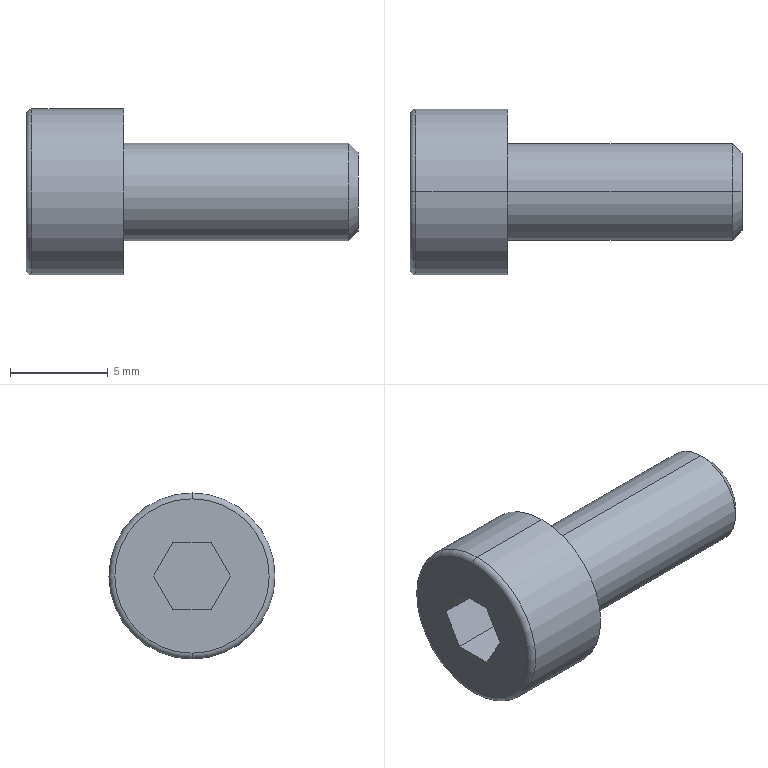Part | SolidWorks | features ICE 1, Revolution 1 | 1 solid | 18 faces | box 17 x 8.5 x 8.5 mm | volume 492.043 mm3 | plane 10 | cylinder 4 | torus 2 | cone 2 | commonest cylinder face diameters 5 x2 8.5 x2
STEP:
#1=CARTESIAN_POINT('',(0.,0.,-3.95));
#2=VERTEX_POINT('',#1);
#3=CARTESIAN_POINT('',(0.,0.,3.95));
#4=VERTEX_POINT('',#3);
#5=CARTESIAN_POINT('',(0.,0.,0.));
#6=DIRECTION('',(1.,0.,0.));
#7=DIRECTION('',(0.,0.,-1.));
#8=AXIS2_PLACEMENT_3D('',#5,#6,#7);
#9=CIRCLE('',#8,3.95);
#10=EDGE_CURVE('',#2,#4,#9,.T.);
#11=ORIENTED_EDGE('',*,*,#10,.T.);
#12=CARTESIAN_POINT('',(0.3,0.,4.25));
#13=VERTEX_POINT('',#12);
#14=CARTESIAN_POINT('',(0.3,0.,3.95));
#15=DIRECTION('',(0.,1.,0.));
#16=DIRECTION('',(0.,0.,1.));
#17=AXIS2_PLACEMENT_3D('',#14,#15,#16);
#18=CIRCLE('',#17,0.3);
#19=EDGE_CURVE('',#4,#13,#18,.T.);
#20=ORIENTED_EDGE('',*,*,#19,.T.);
#21=CARTESIAN_POINT('',(0.3,0.,-4.25));
#22=VERTEX_POINT('',#21);
#23=CARTESIAN_POINT('',(0.3,0.,0.));
#24=DIRECTION('',(1.,0.,0.));
#25=DIRECTION('',(0.,0.,-1.));
#26=AXIS2_PLACEMENT_3D('',#23,#24,#25);
#27=CIRCLE('',#26,4.25);
#28=EDGE_CURVE('',#22,#13,#27,.T.);
#29=ORIENTED_EDGE('',*,*,#28,.F.);
#30=CARTESIAN_POINT('',(0.3,0.,-3.95));
#31=DIRECTION('',(0.,-1.,0.));
#32=DIRECTION('',(0.,0.,-1.));
#33=AXIS2_PLACEMENT_3D('',#30,#31,#32);
#34=CIRCLE('',#33,0.3);
#35=EDGE_CURVE('',#2,#22,#34,.T.);
#36=ORIENTED_EDGE('',*,*,#35,.F.);
#37=EDGE_LOOP('',(#11,#20,#29,#36));
#38=FACE_OUTER_BOUND('',#37,.T.);
#39=CARTESIAN_POINT('',(0.3,0.,0.));
#40=DIRECTION('',(1.,0.,0.));
#41=DIRECTION('',(0.,0.,-1.));
#42=AXIS2_PLACEMENT_3D('',#39,#40,#41);
#43=TOROIDAL_SURFACE('',#42,3.95,0.3);
#44=ADVANCED_FACE('',(#38),#43,.T.);
#45=ORIENTED_EDGE('',*,*,#28,.T.);
#46=CARTESIAN_POINT('',(5.,0.,4.25));
#47=VERTEX_POINT('',#46);
#48=CARTESIAN_POINT('',(0.,0.,4.25));
#49=DIRECTION('',(1.,0.,0.));
#50=VECTOR('',#49,1000.);
#51=LINE('',#48,#50);
#52=EDGE_CURVE('',#13,#47,#51,.T.);
#53=ORIENTED_EDGE('',*,*,#52,.T.);
#54=CARTESIAN_POINT('',(5.,0.,-4.25));
#55=VERTEX_POINT('',#54);
#56=CARTESIAN_POINT('',(5.,0.,0.));
#57=DIRECTION('',(1.,0.,0.));
#58=DIRECTION('',(0.,0.,-1.));
#59=AXIS2_PLACEMENT_3D('',#56,#57,#58);
#60=CIRCLE('',#59,4.25);
#61=EDGE_CURVE('',#55,#47,#60,.T.);
#62=ORIENTED_EDGE('',*,*,#61,.F.);
#63=CARTESIAN_POINT('',(0.,0.,-4.25));
#64=DIRECTION('',(1.,0.,0.));
#65=VECTOR('',#64,1000.);
#66=LINE('',#63,#65);
#67=EDGE_CURVE('',#22,#55,#66,.T.);
#68=ORIENTED_EDGE('',*,*,#67,.F.);
#69=EDGE_LOOP('',(#45,#53,#62,#68));
#70=FACE_OUTER_BOUND('',#69,.T.);
#71=CARTESIAN_POINT('',(0.,0.,0.));
#72=DIRECTION('',(1.,0.,0.));
#73=DIRECTION('',(0.,0.,-1.));
#74=AXIS2_PLACEMENT_3D('',#71,#72,#73);
#75=CYLINDRICAL_SURFACE('',#74,4.25);
#76=ADVANCED_FACE('',(#70),#75,.T.);
#77=CARTESIAN_POINT('',(5.,0.,-2.5));
#78=VERTEX_POINT('',#77);
#79=CARTESIAN_POINT('',(5.,0.,2.5));
#80=VERTEX_POINT('',#79);
#81=CARTESIAN_POINT('',(5.,0.,0.));
#82=DIRECTION('',(1.,0.,0.));
#83=DIRECTION('',(0.,0.,-1.));
#84=AXIS2_PLACEMENT_3D('',#81,#82,#83);
#85=CIRCLE('',#84,2.5);
#86=EDGE_CURVE('',#78,#80,#85,.T.);
#87=ORIENTED_EDGE('',*,*,#86,.T.);
#88=CARTESIAN_POINT('',(16.509,0.,2.5));
#89=VERTEX_POINT('',#88);
#90=CARTESIAN_POINT('',(0.,0.,2.5));
#91=DIRECTION('',(1.,0.,0.));
#92=VECTOR('',#91,1000.);
#93=LINE('',#90,#92);
#94=EDGE_CURVE('',#80,#89,#93,.T.);
#95=ORIENTED_EDGE('',*,*,#94,.T.);
#96=CARTESIAN_POINT('',(16.509,0.,-2.5));
#97=VERTEX_POINT('',#96);
#98=CARTESIAN_POINT('',(16.509,0.,0.));
#99=DIRECTION('',(1.,0.,0.));
#100=DIRECTION('',(0.,0.,-1.));
#101=AXIS2_PLACEMENT_3D('',#98,#99,#100);
#102=CIRCLE('',#101,2.5);
#103=EDGE_CURVE('',#97,#89,#102,.T.);
#104=ORIENTED_EDGE('',*,*,#103,.F.);
#105=CARTESIAN_POINT('',(0.,0.,-2.5));
#106=DIRECTION('',(1.,0.,0.));
#107=VECTOR('',#106,1000.);
#108=LINE('',#105,#107);
#109=EDGE_CURVE('',#78,#97,#108,.T.);
#110=ORIENTED_EDGE('',*,*,#109,.F.);
#111=EDGE_LOOP('',(#87,#95,#104,#110));
#112=FACE_OUTER_BOUND('',#111,.T.);
#113=CARTESIAN_POINT('',(0.,0.,0.));
#114=DIRECTION('',(1.,0.,0.));
#115=DIRECTION('',(0.,0.,-1.));
#116=AXIS2_PLACEMENT_3D('',#113,#114,#115);
#117=CYLINDRICAL_SURFACE('',#116,2.5);
#118=ADVANCED_FACE('',(#112),#117,.T.);
#119=CARTESIAN_POINT('',(17.,0.,-2.01));
#120=VERTEX_POINT('',#119);
#121=CARTESIAN_POINT('',(17.,0.,2.01));
#122=VERTEX_POINT('',#121);
#123=CARTESIAN_POINT('',(17.,0.,0.));
#124=DIRECTION('',(1.,0.,0.));
#125=DIRECTION('',(0.,0.,-1.));
#126=AXIS2_PLACEMENT_3D('',#123,#124,#125);
#127=CIRCLE('',#126,2.01);
#128=EDGE_CURVE('',#120,#122,#127,.T.);
#129=ORIENTED_EDGE('',*,*,#128,.F.);
#130=CARTESIAN_POINT('',(16.509,0.,-2.5));
#131=DIRECTION('',(-0.7071,0.,-0.7071));
#132=VECTOR('',#131,1000.);
#133=LINE('',#130,#132);
#134=EDGE_CURVE('',#120,#97,#133,.T.);
#135=ORIENTED_EDGE('',*,*,#134,.T.);
#136=ORIENTED_EDGE('',*,*,#103,.T.);
#137=CARTESIAN_POINT('',(16.509,0.,2.5));
#138=DIRECTION('',(-0.7071,0.,0.7071));
#139=VECTOR('',#138,1000.);
#140=LINE('',#137,#139);
#141=EDGE_CURVE('',#122,#89,#140,.T.);
#142=ORIENTED_EDGE('',*,*,#141,.F.);
#143=EDGE_LOOP('',(#129,#135,#136,#142));
#144=FACE_OUTER_BOUND('',#143,.T.);
#145=CARTESIAN_POINT('',(16.509,0.,0.));
#146=DIRECTION('',(-1.,0.,0.));
#147=DIRECTION('',(0.,0.,1.));
#148=AXIS2_PLACEMENT_3D('',#145,#146,#147);
#149=CONICAL_SURFACE('',#148,2.5,0.7854);
#150=ADVANCED_FACE('',(#144),#149,.T.);
#151=ORIENTED_EDGE('',*,*,#10,.F.);
#152=CARTESIAN_POINT('',(0.,0.,0.));
#153=DIRECTION('',(1.,0.,0.));
#154=DIRECTION('',(0.,0.,-1.));
#155=AXIS2_PLACEMENT_3D('',#152,#153,#154);
#156=CIRCLE('',#155,3.95);
#157=EDGE_CURVE('',#4,#2,#156,.T.);
#158=ORIENTED_EDGE('',*,*,#157,.F.);
#159=EDGE_LOOP('',(#151,#158));
#160=FACE_OUTER_BOUND('',#159,.T.);
#161=CARTESIAN_POINT('',(0.,0.9815,1.7));
#162=VERTEX_POINT('',#161);
#163=CARTESIAN_POINT('',(0.,-0.9815,1.7));
#164=VERTEX_POINT('',#163);
#165=CARTESIAN_POINT('',(0.,0.9815,1.7));
#166=DIRECTION('',(0.,-1.,0.));
#167=VECTOR('',#166,1000.);
#168=LINE('',#165,#167);
#169=EDGE_CURVE('',#162,#164,#168,.T.);
#170=ORIENTED_EDGE('',*,*,#169,.T.);
#171=CARTESIAN_POINT('',(0.,-1.963,0.));
#172=VERTEX_POINT('',#171);
#173=CARTESIAN_POINT('',(0.,-0.9815,1.7));
#174=DIRECTION('',(0.,-0.5,-0.866));
#175=VECTOR('',#174,1000.);
#176=LINE('',#173,#175);
#177=EDGE_CURVE('',#164,#172,#176,.T.);
#178=ORIENTED_EDGE('',*,*,#177,.T.);
#179=CARTESIAN_POINT('',(0.,-0.9815,-1.7));
#180=VERTEX_POINT('',#179);
#181=CARTESIAN_POINT('',(0.,-1.963,0.));
#182=DIRECTION('',(0.,0.5,-0.866));
#183=VECTOR('',#182,1000.);
#184=LINE('',#181,#183);
#185=EDGE_CURVE('',#172,#180,#184,.T.);
#186=ORIENTED_EDGE('',*,*,#185,.T.);
#187=CARTESIAN_POINT('',(0.,0.9815,-1.7));
#188=VERTEX_POINT('',#187);
#189=CARTESIAN_POINT('',(0.,-0.9815,-1.7));
#190=DIRECTION('',(0.,1.,0.));
#191=VECTOR('',#190,1000.);
#192=LINE('',#189,#191);
#193=EDGE_CURVE('',#180,#188,#192,.T.);
#194=ORIENTED_EDGE('',*,*,#193,.T.);
#195=CARTESIAN_POINT('',(0.,1.963,0.));
#196=VERTEX_POINT('',#195);
#197=CARTESIAN_POINT('',(0.,0.9815,-1.7));
#198=DIRECTION('',(0.,0.5,0.866));
#199=VECTOR('',#198,1000.);
#200=LINE('',#197,#199);
#201=EDGE_CURVE('',#188,#196,#200,.T.);
#202=ORIENTED_EDGE('',*,*,#201,.T.);
#203=CARTESIAN_POINT('',(0.,1.963,0.));
#204=DIRECTION('',(0.,-0.5,0.866));
#205=VECTOR('',#204,1000.);
#206=LINE('',#203,#205);
#207=EDGE_CURVE('',#196,#162,#206,.T.);
#208=ORIENTED_EDGE('',*,*,#207,.T.);
#209=EDGE_LOOP('',(#170,#178,#186,#194,#202,#208));
#210=FACE_BOUND('',#209,.T.);
#211=CARTESIAN_POINT('',(0.,-3.95,0.));
#212=DIRECTION('',(1.,0.,0.));
#213=DIRECTION('',(0.,0.,-1.));
#214=AXIS2_PLACEMENT_3D('',#211,#212,#213);
#215=PLANE('',#214);
#216=ADVANCED_FACE('',(#160,#210),#215,.F.);
#217=CARTESIAN_POINT('',(17.,0.,0.));
#218=DIRECTION('',(1.,0.,0.));
#219=DIRECTION('',(0.,0.,-1.));
#220=AXIS2_PLACEMENT_3D('',#217,#218,#219);
#221=CIRCLE('',#220,2.01);
#222=EDGE_CURVE('',#122,#120,#221,.T.);
#223=ORIENTED_EDGE('',*,*,#222,.T.);
#224=ORIENTED_EDGE('',*,*,#128,.T.);
#225=EDGE_LOOP('',(#223,#224));
#226=FACE_OUTER_BOUND('',#225,.T.);
#227=CARTESIAN_POINT('',(17.,0.,0.));
#228=DIRECTION('',(-1.,0.,0.));
#229=DIRECTION('',(0.,0.,1.));
#230=AXIS2_PLACEMENT_3D('',#227,#228,#229);
#231=PLANE('',#230);
#232=ADVANCED_FACE('',(#226),#231,.F.);
#233=ORIENTED_EDGE('',*,*,#134,.F.);
#234=ORIENTED_EDGE('',*,*,#222,.F.);
#235=ORIENTED_EDGE('',*,*,#141,.T.);
#236=CARTESIAN_POINT('',(16.509,0.,0.));
#237=DIRECTION('',(1.,0.,0.));
#238=DIRECTION('',(0.,0.,-1.));
#239=AXIS2_PLACEMENT_3D('',#236,#237,#238);
#240=CIRCLE('',#239,2.5);
#241=EDGE_CURVE('',#89,#97,#240,.T.);
#242=ORIENTED_EDGE('',*,*,#241,.T.);
#243=EDGE_LOOP('',(#233,#234,#235,#242));
#244=FACE_OUTER_BOUND('',#243,.T.);
#245=CARTESIAN_POINT('',(16.509,0.,0.));
#246=DIRECTION('',(-1.,0.,0.));
#247=DIRECTION('',(0.,0.,1.));
#248=AXIS2_PLACEMENT_3D('',#245,#246,#247);
#249=CONICAL_SURFACE('',#248,2.5,0.7854);
#250=ADVANCED_FACE('',(#244),#249,.T.);
#251=ORIENTED_EDGE('',*,*,#94,.F.);
#252=CARTESIAN_POINT('',(5.,0.,0.));
#253=DIRECTION('',(1.,0.,0.));
#254=DIRECTION('',(0.,0.,-1.));
#255=AXIS2_PLACEMENT_3D('',#252,#253,#254);
#256=CIRCLE('',#255,2.5);
#257=EDGE_CURVE('',#80,#78,#256,.T.);
#258=ORIENTED_EDGE('',*,*,#257,.T.);
#259=ORIENTED_EDGE('',*,*,#109,.T.);
#260=ORIENTED_EDGE('',*,*,#241,.F.);
#261=EDGE_LOOP('',(#251,#258,#259,#260));
#262=FACE_OUTER_BOUND('',#261,.T.);
#263=CARTESIAN_POINT('',(0.,0.,0.));
#264=DIRECTION('',(1.,0.,0.));
#265=DIRECTION('',(0.,0.,-1.));
#266=AXIS2_PLACEMENT_3D('',#263,#264,#265);
#267=CYLINDRICAL_SURFACE('',#266,2.5);
#268=ADVANCED_FACE('',(#262),#267,.T.);
#269=ORIENTED_EDGE('',*,*,#86,.F.);
#270=ORIENTED_EDGE('',*,*,#257,.F.);
#271=EDGE_LOOP('',(#269,#270));
#272=FACE_BOUND('',#271,.T.);
#273=ORIENTED_EDGE('',*,*,#61,.T.);
#274=CARTESIAN_POINT('',(5.,0.,0.));
#275=DIRECTION('',(1.,0.,0.));
#276=DIRECTION('',(0.,0.,-1.));
#277=AXIS2_PLACEMENT_3D('',#274,#275,#276);
#278=CIRCLE('',#277,4.25);
#279=EDGE_CURVE('',#47,#55,#278,.T.);
#280=ORIENTED_EDGE('',*,*,#279,.T.);
#281=EDGE_LOOP('',(#273,#280));
#282=FACE_OUTER_BOUND('',#281,.T.);
#283=CARTESIAN_POINT('',(5.,-2.5,0.));
#284=DIRECTION('',(-1.,0.,0.));
#285=DIRECTION('',(0.,0.,1.));
#286=AXIS2_PLACEMENT_3D('',#283,#284,#285);
#287=PLANE('',#286);
#288=ADVANCED_FACE('',(#272,#282),#287,.F.);
#289=ORIENTED_EDGE('',*,*,#52,.F.);
#290=CARTESIAN_POINT('',(0.3,0.,0.));
#291=DIRECTION('',(1.,0.,0.));
#292=DIRECTION('',(0.,0.,-1.));
#293=AXIS2_PLACEMENT_3D('',#290,#291,#292);
#294=CIRCLE('',#293,4.25);
#295=EDGE_CURVE('',#13,#22,#294,.T.);
#296=ORIENTED_EDGE('',*,*,#295,.T.);
#297=ORIENTED_EDGE('',*,*,#67,.T.);
#298=ORIENTED_EDGE('',*,*,#279,.F.);
#299=EDGE_LOOP('',(#289,#296,#297,#298));
#300=FACE_OUTER_BOUND('',#299,.T.);
#301=CARTESIAN_POINT('',(0.,0.,0.));
#302=DIRECTION('',(1.,0.,0.));
#303=DIRECTION('',(0.,0.,-1.));
#304=AXIS2_PLACEMENT_3D('',#301,#302,#303);
#305=CYLINDRICAL_SURFACE('',#304,4.25);
#306=ADVANCED_FACE('',(#300),#305,.T.);
#307=ORIENTED_EDGE('',*,*,#19,.F.);
#308=ORIENTED_EDGE('',*,*,#157,.T.);
#309=ORIENTED_EDGE('',*,*,#35,.T.);
#310=ORIENTED_EDGE('',*,*,#295,.F.);
#311=EDGE_LOOP('',(#307,#308,#309,#310));
#312=FACE_OUTER_BOUND('',#311,.T.);
#313=CARTESIAN_POINT('',(0.3,0.,0.));
#314=DIRECTION('',(1.,0.,0.));
#315=DIRECTION('',(0.,0.,-1.));
#316=AXIS2_PLACEMENT_3D('',#313,#314,#315);
#317=TOROIDAL_SURFACE('',#316,3.95,0.3);
#318=ADVANCED_FACE('',(#312),#317,.T.);
#319=ORIENTED_EDGE('',*,*,#169,.F.);
#320=CARTESIAN_POINT('',(2.5,0.9815,1.7));
#321=VERTEX_POINT('',#320);
#322=CARTESIAN_POINT('',(2.5,0.9815,1.7));
#323=DIRECTION('',(-1.,0.,0.));
#324=VECTOR('',#323,1000.);
#325=LINE('',#322,#324);
#326=EDGE_CURVE('',#321,#162,#325,.T.);
#327=ORIENTED_EDGE('',*,*,#326,.F.);
#328=CARTESIAN_POINT('',(2.5,-0.9815,1.7));
#329=VERTEX_POINT('',#328);
#330=CARTESIAN_POINT('',(2.5,0.9815,1.7));
#331=DIRECTION('',(0.,-1.,0.));
#332=VECTOR('',#331,1000.);
#333=LINE('',#330,#332);
#334=EDGE_CURVE('',#321,#329,#333,.T.);
#335=ORIENTED_EDGE('',*,*,#334,.T.);
#336=CARTESIAN_POINT('',(2.5,-0.9815,1.7));
#337=DIRECTION('',(-1.,0.,0.));
#338=VECTOR('',#337,1000.);
#339=LINE('',#336,#338);
#340=EDGE_CURVE('',#329,#164,#339,.T.);
#341=ORIENTED_EDGE('',*,*,#340,.T.);
#342=EDGE_LOOP('',(#319,#327,#335,#341));
#343=FACE_OUTER_BOUND('',#342,.T.);
#344=CARTESIAN_POINT('',(2.5,0.9815,1.7));
#345=DIRECTION('',(0.,0.,-1.));
#346=DIRECTION('',(-1.,0.,0.));
#347=AXIS2_PLACEMENT_3D('',#344,#345,#346);
#348=PLANE('',#347);
#349=ADVANCED_FACE('',(#343),#348,.T.);
#350=ORIENTED_EDGE('',*,*,#177,.F.);
#351=ORIENTED_EDGE('',*,*,#340,.F.);
#352=CARTESIAN_POINT('',(2.5,-1.963,0.));
#353=VERTEX_POINT('',#352);
#354=CARTESIAN_POINT('',(2.5,-0.9815,1.7));
#355=DIRECTION('',(0.,-0.5,-0.866));
#356=VECTOR('',#355,1000.);
#357=LINE('',#354,#356);
#358=EDGE_CURVE('',#329,#353,#357,.T.);
#359=ORIENTED_EDGE('',*,*,#358,.T.);
#360=CARTESIAN_POINT('',(2.5,-1.963,0.));
#361=DIRECTION('',(-1.,0.,0.));
#362=VECTOR('',#361,1000.);
#363=LINE('',#360,#362);
#364=EDGE_CURVE('',#353,#172,#363,.T.);
#365=ORIENTED_EDGE('',*,*,#364,.T.);
#366=EDGE_LOOP('',(#350,#351,#359,#365));
#367=FACE_OUTER_BOUND('',#366,.T.);
#368=CARTESIAN_POINT('',(2.5,-0.9815,1.7));
#369=DIRECTION('',(0.,0.866,-0.5));
#370=DIRECTION('',(0.,0.5,0.866));
#371=AXIS2_PLACEMENT_3D('',#368,#369,#370);
#372=PLANE('',#371);
#373=ADVANCED_FACE('',(#367),#372,.T.);
#374=ORIENTED_EDGE('',*,*,#185,.F.);
#375=ORIENTED_EDGE('',*,*,#364,.F.);
#376=CARTESIAN_POINT('',(2.5,-0.9815,-1.7));
#377=VERTEX_POINT('',#376);
#378=CARTESIAN_POINT('',(2.5,-1.963,0.));
#379=DIRECTION('',(0.,0.5,-0.866));
#380=VECTOR('',#379,1000.);
#381=LINE('',#378,#380);
#382=EDGE_CURVE('',#353,#377,#381,.T.);
#383=ORIENTED_EDGE('',*,*,#382,.T.);
#384=CARTESIAN_POINT('',(2.5,-0.9815,-1.7));
#385=DIRECTION('',(-1.,0.,0.));
#386=VECTOR('',#385,1000.);
#387=LINE('',#384,#386);
#388=EDGE_CURVE('',#377,#180,#387,.T.);
#389=ORIENTED_EDGE('',*,*,#388,.T.);
#390=EDGE_LOOP('',(#374,#375,#383,#389));
#391=FACE_OUTER_BOUND('',#390,.T.);
#392=CARTESIAN_POINT('',(2.5,-1.963,0.));
#393=DIRECTION('',(0.,0.866,0.5));
#394=DIRECTION('',(0.,-0.5,0.866));
#395=AXIS2_PLACEMENT_3D('',#392,#393,#394);
#396=PLANE('',#395);
#397=ADVANCED_FACE('',(#391),#396,.T.);
#398=ORIENTED_EDGE('',*,*,#193,.F.);
#399=ORIENTED_EDGE('',*,*,#388,.F.);
#400=CARTESIAN_POINT('',(2.5,0.9815,-1.7));
#401=VERTEX_POINT('',#400);
#402=CARTESIAN_POINT('',(2.5,-0.9815,-1.7));
#403=DIRECTION('',(0.,1.,0.));
#404=VECTOR('',#403,1000.);
#405=LINE('',#402,#404);
#406=EDGE_CURVE('',#377,#401,#405,.T.);
#407=ORIENTED_EDGE('',*,*,#406,.T.);
#408=CARTESIAN_POINT('',(2.5,0.9815,-1.7));
#409=DIRECTION('',(-1.,0.,0.));
#410=VECTOR('',#409,1000.);
#411=LINE('',#408,#410);
#412=EDGE_CURVE('',#401,#188,#411,.T.);
#413=ORIENTED_EDGE('',*,*,#412,.T.);
#414=EDGE_LOOP('',(#398,#399,#407,#413));
#415=FACE_OUTER_BOUND('',#414,.T.);
#416=CARTESIAN_POINT('',(2.5,-0.9815,-1.7));
#417=DIRECTION('',(0.,0.,1.));
#418=DIRECTION('',(1.,0.,0.));
#419=AXIS2_PLACEMENT_3D('',#416,#417,#418);
#420=PLANE('',#419);
#421=ADVANCED_FACE('',(#415),#420,.T.);
#422=ORIENTED_EDGE('',*,*,#201,.F.);
#423=ORIENTED_EDGE('',*,*,#412,.F.);
#424=CARTESIAN_POINT('',(2.5,1.963,0.));
#425=VERTEX_POINT('',#424);
#426=CARTESIAN_POINT('',(2.5,0.9815,-1.7));
#427=DIRECTION('',(0.,0.5,0.866));
#428=VECTOR('',#427,1000.);
#429=LINE('',#426,#428);
#430=EDGE_CURVE('',#401,#425,#429,.T.);
#431=ORIENTED_EDGE('',*,*,#430,.T.);
#432=CARTESIAN_POINT('',(2.5,1.963,0.));
#433=DIRECTION('',(-1.,0.,0.));
#434=VECTOR('',#433,1000.);
#435=LINE('',#432,#434);
#436=EDGE_CURVE('',#425,#196,#435,.T.);
#437=ORIENTED_EDGE('',*,*,#436,.T.);
#438=EDGE_LOOP('',(#422,#423,#431,#437));
#439=FACE_OUTER_BOUND('',#438,.T.);
#440=CARTESIAN_POINT('',(2.5,0.9815,-1.7));
#441=DIRECTION('',(0.,-0.866,0.5));
#442=DIRECTION('',(0.,-0.5,-0.866));
#443=AXIS2_PLACEMENT_3D('',#440,#441,#442);
#444=PLANE('',#443);
#445=ADVANCED_FACE('',(#439),#444,.T.);
#446=ORIENTED_EDGE('',*,*,#207,.F.);
#447=ORIENTED_EDGE('',*,*,#436,.F.);
#448=CARTESIAN_POINT('',(2.5,1.963,0.));
#449=DIRECTION('',(0.,-0.5,0.866));
#450=VECTOR('',#449,1000.);
#451=LINE('',#448,#450);
#452=EDGE_CURVE('',#425,#321,#451,.T.);
#453=ORIENTED_EDGE('',*,*,#452,.T.);
#454=ORIENTED_EDGE('',*,*,#326,.T.);
#455=EDGE_LOOP('',(#446,#447,#453,#454));
#456=FACE_OUTER_BOUND('',#455,.T.);
#457=CARTESIAN_POINT('',(2.5,1.963,0.));
#458=DIRECTION('',(0.,-0.866,-0.5));
#459=DIRECTION('',(0.,0.5,-0.866));
#460=AXIS2_PLACEMENT_3D('',#457,#458,#459);
#461=PLANE('',#460);
#462=ADVANCED_FACE('',(#456),#461,.T.);
#463=ORIENTED_EDGE('',*,*,#334,.F.);
#464=ORIENTED_EDGE('',*,*,#452,.F.);
#465=ORIENTED_EDGE('',*,*,#430,.F.);
#466=ORIENTED_EDGE('',*,*,#406,.F.);
#467=ORIENTED_EDGE('',*,*,#382,.F.);
#468=ORIENTED_EDGE('',*,*,#358,.F.);
#469=EDGE_LOOP('',(#463,#464,#465,#466,#467,#468));
#470=FACE_OUTER_BOUND('',#469,.T.);
#471=CARTESIAN_POINT('',(2.5,0.,0.));
#472=DIRECTION('',(1.,0.,0.));
#473=DIRECTION('',(0.,0.,-1.));
#474=AXIS2_PLACEMENT_3D('',#471,#472,#473);
#475=PLANE('',#474);
#476=ADVANCED_FACE('',(#470),#475,.F.);
#477=CLOSED_SHELL('',(#44,#76,#118,#150,#216,#232,#250,#268,#288,#306,#318,#349,#373,#397,#421,#445,#462,#476));
#478=MANIFOLD_SOLID_BREP('',#477);
#479=CARTESIAN_POINT('',(0.,0.,0.));
#480=DIRECTION('',(0.,0.,1.));
#481=DIRECTION('',(1.,0.,0.));
#482=AXIS2_PLACEMENT_3D('',#479,#480,#481);
#483=(LENGTH_UNIT()NAMED_UNIT(*)SI_UNIT(.MILLI.,.METRE.));
#484=UNCERTAINTY_MEASURE_WITH_UNIT(LENGTH_MEASURE(0.00001),#483,'','');
#485=(NAMED_UNIT(*)PLANE_ANGLE_UNIT()SI_UNIT($,.RADIAN.));
#486=(NAMED_UNIT(*)SI_UNIT($,.STERADIAN.)SOLID_ANGLE_UNIT());
#487=(GEOMETRIC_REPRESENTATION_CONTEXT(3)GLOBAL_UNCERTAINTY_ASSIGNED_CONTEXT((#484))GLOBAL_UNIT_ASSIGNED_CONTEXT((#483,#485,#486))REPRESENTATION_CONTEXT('',''));
#488=ADVANCED_BREP_SHAPE_REPRESENTATION('',(#478,#482),#487);